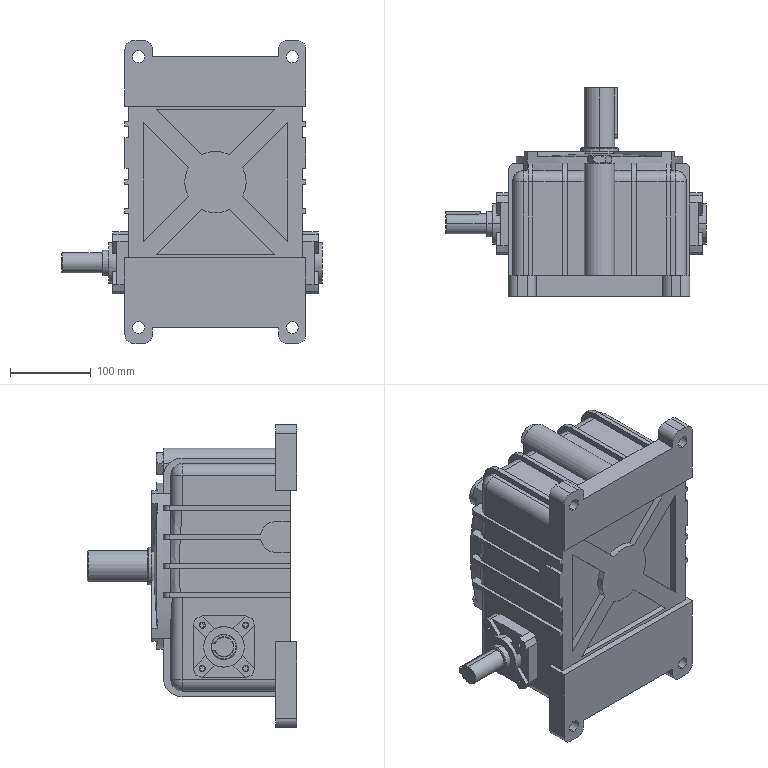Part | SolidWorks | features ICE 22, DeleteBody 4, Fillet 4, LPattern 3, MirrorSolid 3, Chamfer 2, CirPattern 2, Revolution 2, CombineBodies 1, Extrusion 1, MirrorPattern 1, RevCut 1 | 3 solids | 536 faces | box 322 x 259 x 375 mm | volume 10630129 mm3 | plane 336 | cylinder 135 | cone 31 | torus 24 | spline 6 | sphere 4 | commonest cylinder face diameters 28.125 x20 7.268 x16 7.65 x16 76 x10 46.24 x9 14.063 x8